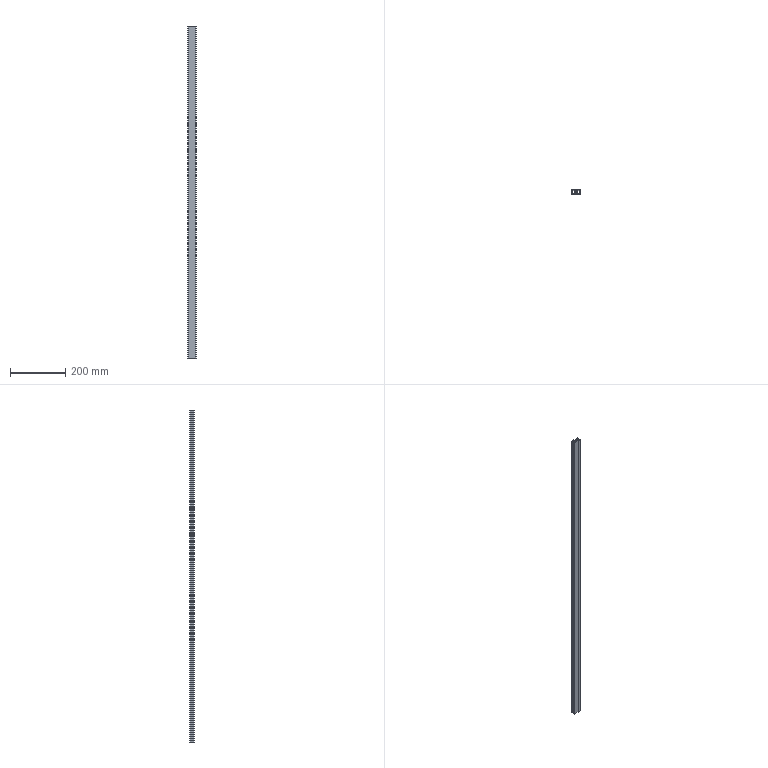Part | SolidWorks | features BaseBody 1, MoveFace 1 | 1 solid | 53 faces | box 30 x 15 x 1200 mm | volume 289403 mm3 | plane 38 | cylinder 15 | commonest cylinder face diameters 1 x6 5 x5 2 x4